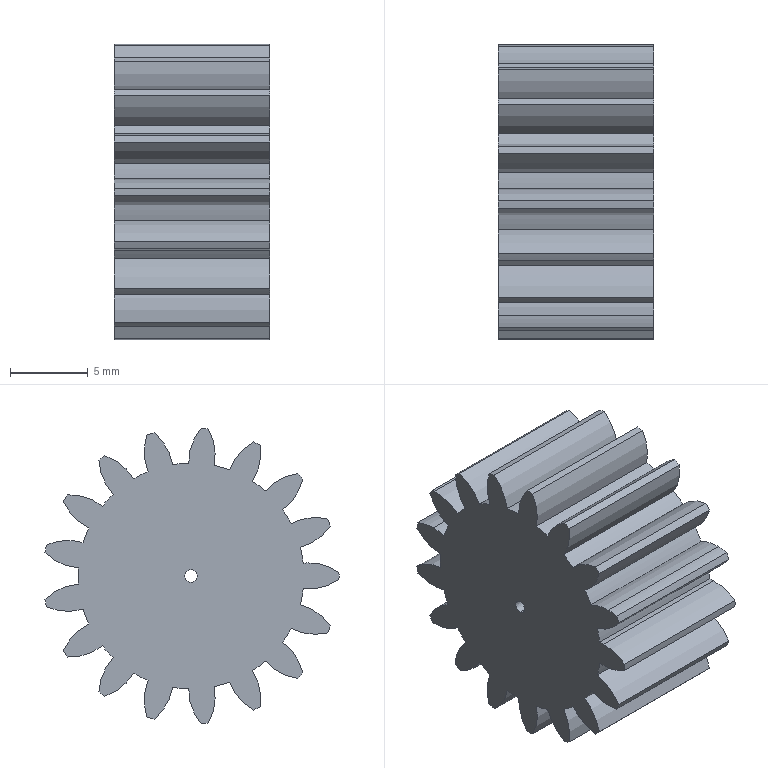Part | STEP file | spur gear_iso_ISO - Spur gear 1M 17T 20PA 10FW ---S17A75H50L0.8N | 1 solid | 76 faces | box 10 x 18.879 x 18.957 mm | volume 2165 mm3 | cylinder 74 | plane 2 | commonest cylinder face diameters 6.8 x38 14.498 x17 19 x17 0.8 x2